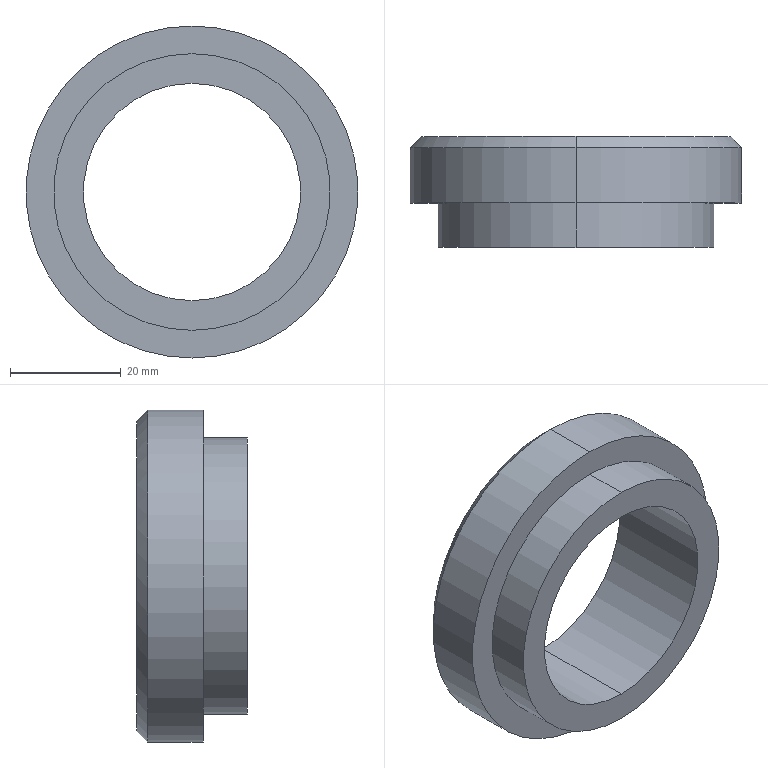Part | SolidWorks | features Chamfer 1, HoleWzd 1, Revolution 1 | 1 solid | 11 faces | box 60 x 20 x 60 mm | volume 25069 mm3 | cylinder 6 | plane 3 | cone 2 | commonest cylinder face diameters 39.25 x2 50 x2 60 x2
STEP:
#1=CARTESIAN_POINT('',(0.,0.,28.));
#2=VERTEX_POINT('',#1);
#3=CARTESIAN_POINT('',(0.,0.,-28.));
#4=VERTEX_POINT('',#3);
#5=CARTESIAN_POINT('',(0.,0.,0.));
#6=DIRECTION('',(0.,1.,0.));
#7=DIRECTION('',(0.,0.,1.));
#8=AXIS2_PLACEMENT_3D('',#5,#6,#7);
#9=CIRCLE('',#8,28.);
#10=EDGE_CURVE('',#2,#4,#9,.T.);
#11=ORIENTED_EDGE('',*,*,#10,.F.);
#12=CARTESIAN_POINT('',(0.,-2.,30.));
#13=VERTEX_POINT('',#12);
#14=CARTESIAN_POINT('',(0.,-2.,30.));
#15=DIRECTION('',(0.,-0.7071,0.7071));
#16=VECTOR('',#15,1000.);
#17=LINE('',#14,#16);
#18=EDGE_CURVE('',#2,#13,#17,.T.);
#19=ORIENTED_EDGE('',*,*,#18,.T.);
#20=CARTESIAN_POINT('',(0.,-2.,-30.));
#21=VERTEX_POINT('',#20);
#22=CARTESIAN_POINT('',(0.,-2.,0.));
#23=DIRECTION('',(0.,-1.,0.));
#24=DIRECTION('',(0.,0.,1.));
#25=AXIS2_PLACEMENT_3D('',#22,#23,#24);
#26=CIRCLE('',#25,30.);
#27=EDGE_CURVE('',#21,#13,#26,.T.);
#28=ORIENTED_EDGE('',*,*,#27,.F.);
#29=CARTESIAN_POINT('',(0.,-2.,-30.));
#30=DIRECTION('',(0.,-0.7071,-0.7071));
#31=VECTOR('',#30,1000.);
#32=LINE('',#29,#31);
#33=EDGE_CURVE('',#4,#21,#32,.T.);
#34=ORIENTED_EDGE('',*,*,#33,.F.);
#35=EDGE_LOOP('',(#11,#19,#28,#34));
#36=FACE_OUTER_BOUND('',#35,.T.);
#37=CARTESIAN_POINT('',(0.,-2.,0.));
#38=DIRECTION('',(0.,-1.,0.));
#39=DIRECTION('',(0.,0.,-1.));
#40=AXIS2_PLACEMENT_3D('',#37,#38,#39);
#41=CONICAL_SURFACE('',#40,30.,0.7854);
#42=ADVANCED_FACE('',(#36),#41,.T.);
#43=CARTESIAN_POINT('',(0.,-20.,19.625));
#44=VERTEX_POINT('',#43);
#45=CARTESIAN_POINT('',(0.,-20.,-19.625));
#46=VERTEX_POINT('',#45);
#47=CARTESIAN_POINT('',(0.,-20.,0.));
#48=DIRECTION('',(0.,-1.,0.));
#49=DIRECTION('',(0.,0.,-1.));
#50=AXIS2_PLACEMENT_3D('',#47,#48,#49);
#51=CIRCLE('',#50,19.625);
#52=EDGE_CURVE('',#44,#46,#51,.T.);
#53=ORIENTED_EDGE('',*,*,#52,.T.);
#54=CARTESIAN_POINT('',(0.,0.,-19.625));
#55=VERTEX_POINT('',#54);
#56=CARTESIAN_POINT('',(0.,0.,-19.625));
#57=DIRECTION('',(0.,1.,0.));
#58=VECTOR('',#57,1000.);
#59=LINE('',#56,#58);
#60=EDGE_CURVE('',#46,#55,#59,.T.);
#61=ORIENTED_EDGE('',*,*,#60,.T.);
#62=CARTESIAN_POINT('',(0.,0.,19.625));
#63=VERTEX_POINT('',#62);
#64=CARTESIAN_POINT('',(0.,0.,0.));
#65=DIRECTION('',(0.,1.,0.));
#66=DIRECTION('',(0.,0.,1.));
#67=AXIS2_PLACEMENT_3D('',#64,#65,#66);
#68=CIRCLE('',#67,19.625);
#69=EDGE_CURVE('',#55,#63,#68,.T.);
#70=ORIENTED_EDGE('',*,*,#69,.T.);
#71=CARTESIAN_POINT('',(0.,0.,19.625));
#72=DIRECTION('',(0.,1.,0.));
#73=VECTOR('',#72,1000.);
#74=LINE('',#71,#73);
#75=EDGE_CURVE('',#44,#63,#74,.T.);
#76=ORIENTED_EDGE('',*,*,#75,.F.);
#77=EDGE_LOOP('',(#53,#61,#70,#76));
#78=FACE_OUTER_BOUND('',#77,.T.);
#79=CARTESIAN_POINT('',(0.,0.,0.));
#80=DIRECTION('',(0.,1.,0.));
#81=DIRECTION('',(0.,0.,1.));
#82=AXIS2_PLACEMENT_3D('',#79,#80,#81);
#83=CYLINDRICAL_SURFACE('',#82,19.625);
#84=ADVANCED_FACE('',(#78),#83,.F.);
#85=CARTESIAN_POINT('',(0.,-12.,-25.));
#86=VERTEX_POINT('',#85);
#87=CARTESIAN_POINT('',(0.,-12.,25.));
#88=VERTEX_POINT('',#87);
#89=CARTESIAN_POINT('',(0.,-12.,0.));
#90=DIRECTION('',(0.,-1.,0.));
#91=DIRECTION('',(0.,0.,-1.));
#92=AXIS2_PLACEMENT_3D('',#89,#90,#91);
#93=CIRCLE('',#92,25.);
#94=EDGE_CURVE('',#86,#88,#93,.T.);
#95=ORIENTED_EDGE('',*,*,#94,.T.);
#96=CARTESIAN_POINT('',(0.,-20.,25.));
#97=VERTEX_POINT('',#96);
#98=CARTESIAN_POINT('',(0.,-20.,25.));
#99=DIRECTION('',(0.,-1.,0.));
#100=VECTOR('',#99,1000.);
#101=LINE('',#98,#100);
#102=EDGE_CURVE('',#88,#97,#101,.T.);
#103=ORIENTED_EDGE('',*,*,#102,.T.);
#104=CARTESIAN_POINT('',(0.,-20.,-25.));
#105=VERTEX_POINT('',#104);
#106=CARTESIAN_POINT('',(0.,-20.,0.));
#107=DIRECTION('',(0.,-1.,0.));
#108=DIRECTION('',(0.,0.,-1.));
#109=AXIS2_PLACEMENT_3D('',#106,#107,#108);
#110=CIRCLE('',#109,25.);
#111=EDGE_CURVE('',#105,#97,#110,.T.);
#112=ORIENTED_EDGE('',*,*,#111,.F.);
#113=CARTESIAN_POINT('',(0.,-20.,-25.));
#114=DIRECTION('',(0.,-1.,0.));
#115=VECTOR('',#114,1000.);
#116=LINE('',#113,#115);
#117=EDGE_CURVE('',#86,#105,#116,.T.);
#118=ORIENTED_EDGE('',*,*,#117,.F.);
#119=EDGE_LOOP('',(#95,#103,#112,#118));
#120=FACE_OUTER_BOUND('',#119,.T.);
#121=CARTESIAN_POINT('',(0.,-20.,0.));
#122=DIRECTION('',(0.,-1.,0.));
#123=DIRECTION('',(0.,0.,-1.));
#124=AXIS2_PLACEMENT_3D('',#121,#122,#123);
#125=CYLINDRICAL_SURFACE('',#124,25.);
#126=ADVANCED_FACE('',(#120),#125,.T.);
#127=ORIENTED_EDGE('',*,*,#27,.T.);
#128=CARTESIAN_POINT('',(0.,-12.,30.));
#129=VERTEX_POINT('',#128);
#130=CARTESIAN_POINT('',(0.,-20.,30.));
#131=DIRECTION('',(0.,-1.,0.));
#132=VECTOR('',#131,1000.);
#133=LINE('',#130,#132);
#134=EDGE_CURVE('',#13,#129,#133,.T.);
#135=ORIENTED_EDGE('',*,*,#134,.T.);
#136=CARTESIAN_POINT('',(0.,-12.,-30.));
#137=VERTEX_POINT('',#136);
#138=CARTESIAN_POINT('',(0.,-12.,0.));
#139=DIRECTION('',(0.,-1.,0.));
#140=DIRECTION('',(0.,0.,-1.));
#141=AXIS2_PLACEMENT_3D('',#138,#139,#140);
#142=CIRCLE('',#141,30.);
#143=EDGE_CURVE('',#137,#129,#142,.T.);
#144=ORIENTED_EDGE('',*,*,#143,.F.);
#145=CARTESIAN_POINT('',(0.,-20.,-30.));
#146=DIRECTION('',(0.,-1.,0.));
#147=VECTOR('',#146,1000.);
#148=LINE('',#145,#147);
#149=EDGE_CURVE('',#21,#137,#148,.T.);
#150=ORIENTED_EDGE('',*,*,#149,.F.);
#151=EDGE_LOOP('',(#127,#135,#144,#150));
#152=FACE_OUTER_BOUND('',#151,.T.);
#153=CARTESIAN_POINT('',(0.,-20.,0.));
#154=DIRECTION('',(0.,-1.,0.));
#155=DIRECTION('',(0.,0.,-1.));
#156=AXIS2_PLACEMENT_3D('',#153,#154,#155);
#157=CYLINDRICAL_SURFACE('',#156,30.);
#158=ADVANCED_FACE('',(#152),#157,.T.);
#159=CARTESIAN_POINT('',(0.,0.,0.));
#160=DIRECTION('',(0.,1.,0.));
#161=DIRECTION('',(0.,0.,1.));
#162=AXIS2_PLACEMENT_3D('',#159,#160,#161);
#163=CIRCLE('',#162,28.);
#164=EDGE_CURVE('',#4,#2,#163,.T.);
#165=ORIENTED_EDGE('',*,*,#164,.T.);
#166=ORIENTED_EDGE('',*,*,#10,.T.);
#167=EDGE_LOOP('',(#165,#166));
#168=FACE_OUTER_BOUND('',#167,.T.);
#169=CARTESIAN_POINT('',(0.,0.,0.));
#170=DIRECTION('',(0.,1.,0.));
#171=DIRECTION('',(0.,0.,1.));
#172=AXIS2_PLACEMENT_3D('',#169,#170,#171);
#173=CIRCLE('',#172,19.625);
#174=EDGE_CURVE('',#63,#55,#173,.T.);
#175=ORIENTED_EDGE('',*,*,#174,.F.);
#176=ORIENTED_EDGE('',*,*,#69,.F.);
#177=EDGE_LOOP('',(#175,#176));
#178=FACE_BOUND('',#177,.T.);
#179=CARTESIAN_POINT('',(0.,0.,0.));
#180=DIRECTION('',(0.,1.,0.));
#181=DIRECTION('',(0.,0.,1.));
#182=AXIS2_PLACEMENT_3D('',#179,#180,#181);
#183=PLANE('',#182);
#184=ADVANCED_FACE('',(#168,#178),#183,.T.);
#185=ORIENTED_EDGE('',*,*,#134,.F.);
#186=CARTESIAN_POINT('',(0.,-2.,0.));
#187=DIRECTION('',(0.,-1.,0.));
#188=DIRECTION('',(0.,0.,1.));
#189=AXIS2_PLACEMENT_3D('',#186,#187,#188);
#190=CIRCLE('',#189,30.);
#191=EDGE_CURVE('',#13,#21,#190,.T.);
#192=ORIENTED_EDGE('',*,*,#191,.T.);
#193=ORIENTED_EDGE('',*,*,#149,.T.);
#194=CARTESIAN_POINT('',(0.,-12.,0.));
#195=DIRECTION('',(0.,-1.,0.));
#196=DIRECTION('',(0.,0.,-1.));
#197=AXIS2_PLACEMENT_3D('',#194,#195,#196);
#198=CIRCLE('',#197,30.);
#199=EDGE_CURVE('',#129,#137,#198,.T.);
#200=ORIENTED_EDGE('',*,*,#199,.F.);
#201=EDGE_LOOP('',(#185,#192,#193,#200));
#202=FACE_OUTER_BOUND('',#201,.T.);
#203=CARTESIAN_POINT('',(0.,-20.,0.));
#204=DIRECTION('',(0.,-1.,0.));
#205=DIRECTION('',(0.,0.,-1.));
#206=AXIS2_PLACEMENT_3D('',#203,#204,#205);
#207=CYLINDRICAL_SURFACE('',#206,30.);
#208=ADVANCED_FACE('',(#202),#207,.T.);
#209=ORIENTED_EDGE('',*,*,#143,.T.);
#210=ORIENTED_EDGE('',*,*,#199,.T.);
#211=EDGE_LOOP('',(#209,#210));
#212=FACE_OUTER_BOUND('',#211,.T.);
#213=ORIENTED_EDGE('',*,*,#94,.F.);
#214=CARTESIAN_POINT('',(0.,-12.,0.));
#215=DIRECTION('',(0.,-1.,0.));
#216=DIRECTION('',(0.,0.,-1.));
#217=AXIS2_PLACEMENT_3D('',#214,#215,#216);
#218=CIRCLE('',#217,25.);
#219=EDGE_CURVE('',#88,#86,#218,.T.);
#220=ORIENTED_EDGE('',*,*,#219,.F.);
#221=EDGE_LOOP('',(#213,#220));
#222=FACE_BOUND('',#221,.T.);
#223=CARTESIAN_POINT('',(30.,-12.,0.));
#224=DIRECTION('',(0.,-1.,0.));
#225=DIRECTION('',(0.,0.,-1.));
#226=AXIS2_PLACEMENT_3D('',#223,#224,#225);
#227=PLANE('',#226);
#228=ADVANCED_FACE('',(#212,#222),#227,.T.);
#229=ORIENTED_EDGE('',*,*,#102,.F.);
#230=ORIENTED_EDGE('',*,*,#219,.T.);
#231=ORIENTED_EDGE('',*,*,#117,.T.);
#232=CARTESIAN_POINT('',(0.,-20.,0.));
#233=DIRECTION('',(0.,-1.,0.));
#234=DIRECTION('',(0.,0.,-1.));
#235=AXIS2_PLACEMENT_3D('',#232,#233,#234);
#236=CIRCLE('',#235,25.);
#237=EDGE_CURVE('',#97,#105,#236,.T.);
#238=ORIENTED_EDGE('',*,*,#237,.F.);
#239=EDGE_LOOP('',(#229,#230,#231,#238));
#240=FACE_OUTER_BOUND('',#239,.T.);
#241=CARTESIAN_POINT('',(0.,-20.,0.));
#242=DIRECTION('',(0.,-1.,0.));
#243=DIRECTION('',(0.,0.,-1.));
#244=AXIS2_PLACEMENT_3D('',#241,#242,#243);
#245=CYLINDRICAL_SURFACE('',#244,25.);
#246=ADVANCED_FACE('',(#240),#245,.T.);
#247=ORIENTED_EDGE('',*,*,#52,.F.);
#248=CARTESIAN_POINT('',(0.,-20.,0.));
#249=DIRECTION('',(0.,-1.,0.));
#250=DIRECTION('',(0.,0.,-1.));
#251=AXIS2_PLACEMENT_3D('',#248,#249,#250);
#252=CIRCLE('',#251,19.625);
#253=EDGE_CURVE('',#46,#44,#252,.T.);
#254=ORIENTED_EDGE('',*,*,#253,.F.);
#255=EDGE_LOOP('',(#247,#254));
#256=FACE_BOUND('',#255,.T.);
#257=ORIENTED_EDGE('',*,*,#111,.T.);
#258=ORIENTED_EDGE('',*,*,#237,.T.);
#259=EDGE_LOOP('',(#257,#258));
#260=FACE_OUTER_BOUND('',#259,.T.);
#261=CARTESIAN_POINT('',(25.,-20.,0.));
#262=DIRECTION('',(0.,-1.,0.));
#263=DIRECTION('',(0.,0.,-1.));
#264=AXIS2_PLACEMENT_3D('',#261,#262,#263);
#265=PLANE('',#264);
#266=ADVANCED_FACE('',(#256,#260),#265,.T.);
#267=ORIENTED_EDGE('',*,*,#60,.F.);
#268=ORIENTED_EDGE('',*,*,#253,.T.);
#269=ORIENTED_EDGE('',*,*,#75,.T.);
#270=ORIENTED_EDGE('',*,*,#174,.T.);
#271=EDGE_LOOP('',(#267,#268,#269,#270));
#272=FACE_OUTER_BOUND('',#271,.T.);
#273=CARTESIAN_POINT('',(0.,0.,0.));
#274=DIRECTION('',(0.,1.,0.));
#275=DIRECTION('',(0.,0.,1.));
#276=AXIS2_PLACEMENT_3D('',#273,#274,#275);
#277=CYLINDRICAL_SURFACE('',#276,19.625);
#278=ADVANCED_FACE('',(#272),#277,.F.);
#279=ORIENTED_EDGE('',*,*,#18,.F.);
#280=ORIENTED_EDGE('',*,*,#164,.F.);
#281=ORIENTED_EDGE('',*,*,#33,.T.);
#282=ORIENTED_EDGE('',*,*,#191,.F.);
#283=EDGE_LOOP('',(#279,#280,#281,#282));
#284=FACE_OUTER_BOUND('',#283,.T.);
#285=CARTESIAN_POINT('',(0.,-2.,0.));
#286=DIRECTION('',(0.,-1.,0.));
#287=DIRECTION('',(0.,0.,-1.));
#288=AXIS2_PLACEMENT_3D('',#285,#286,#287);
#289=CONICAL_SURFACE('',#288,30.,0.7854);
#290=ADVANCED_FACE('',(#284),#289,.T.);
#291=CLOSED_SHELL('',(#42,#84,#126,#158,#184,#208,#228,#246,#266,#278,#290));
#292=MANIFOLD_SOLID_BREP('',#291);
#293=CARTESIAN_POINT('',(0.,0.,0.));
#294=DIRECTION('',(0.,0.,1.));
#295=DIRECTION('',(1.,0.,0.));
#296=AXIS2_PLACEMENT_3D('',#293,#294,#295);
#297=(LENGTH_UNIT()NAMED_UNIT(*)SI_UNIT(.MILLI.,.METRE.));
#298=UNCERTAINTY_MEASURE_WITH_UNIT(LENGTH_MEASURE(0.00001),#297,'','');
#299=(NAMED_UNIT(*)PLANE_ANGLE_UNIT()SI_UNIT($,.RADIAN.));
#300=(NAMED_UNIT(*)SI_UNIT($,.STERADIAN.)SOLID_ANGLE_UNIT());
#301=(GEOMETRIC_REPRESENTATION_CONTEXT(3)GLOBAL_UNCERTAINTY_ASSIGNED_CONTEXT((#298))GLOBAL_UNIT_ASSIGNED_CONTEXT((#297,#299,#300))REPRESENTATION_CONTEXT('',''));
#302=ADVANCED_BREP_SHAPE_REPRESENTATION('',(#292,#296),#301);